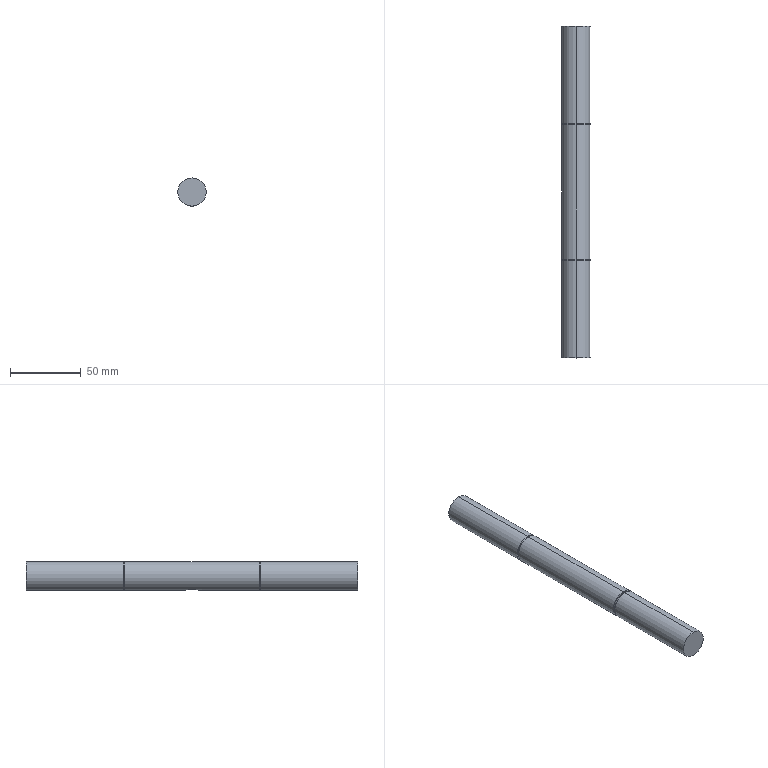Part | SolidWorks | features ICE 3, Chamfer 1, Extrusion 1 | 1 solid | 21 faces | box 20 x 235 x 20 mm | volume 73572 mm3 | cylinder 12 | plane 9 | commonest cylinder face diameters 20 x6 19 x4 6 x2
STEP:
#1=CARTESIAN_POINT('',(0.,235.,10.));
#2=VERTEX_POINT('',#1);
#3=CARTESIAN_POINT('',(0.,235.,-10.));
#4=VERTEX_POINT('',#3);
#5=CARTESIAN_POINT('',(0.,235.,0.));
#6=DIRECTION('',(0.,1.,0.));
#7=DIRECTION('',(0.,0.,1.));
#8=AXIS2_PLACEMENT_3D('',#5,#6,#7);
#9=CIRCLE('',#8,10.);
#10=EDGE_CURVE('',#2,#4,#9,.T.);
#11=ORIENTED_EDGE('',*,*,#10,.F.);
#12=CARTESIAN_POINT('',(0.,166.3,10.));
#13=VERTEX_POINT('',#12);
#14=CARTESIAN_POINT('',(0.,235.,10.));
#15=DIRECTION('',(0.,-1.,0.));
#16=VECTOR('',#15,1000.);
#17=LINE('',#14,#16);
#18=EDGE_CURVE('',#2,#13,#17,.T.);
#19=ORIENTED_EDGE('',*,*,#18,.T.);
#20=CARTESIAN_POINT('',(0.,166.3,-10.));
#21=VERTEX_POINT('',#20);
#22=CARTESIAN_POINT('',(0.,166.3,0.));
#23=DIRECTION('',(0.,1.,0.));
#24=DIRECTION('',(0.,0.,1.));
#25=AXIS2_PLACEMENT_3D('',#22,#23,#24);
#26=CIRCLE('',#25,10.);
#27=EDGE_CURVE('',#13,#21,#26,.T.);
#28=ORIENTED_EDGE('',*,*,#27,.T.);
#29=CARTESIAN_POINT('',(0.,235.,-10.));
#30=DIRECTION('',(0.,-1.,0.));
#31=VECTOR('',#30,1000.);
#32=LINE('',#29,#31);
#33=EDGE_CURVE('',#4,#21,#32,.T.);
#34=ORIENTED_EDGE('',*,*,#33,.F.);
#35=EDGE_LOOP('',(#11,#19,#28,#34));
#36=FACE_OUTER_BOUND('',#35,.T.);
#37=CARTESIAN_POINT('',(0.,235.,0.));
#38=DIRECTION('',(0.,-1.,0.));
#39=DIRECTION('',(0.,0.,-1.));
#40=AXIS2_PLACEMENT_3D('',#37,#38,#39);
#41=CYLINDRICAL_SURFACE('',#40,10.);
#42=ADVANCED_FACE('',(#36),#41,.T.);
#43=CARTESIAN_POINT('',(0.,166.3,9.5));
#44=VERTEX_POINT('',#43);
#45=CARTESIAN_POINT('',(0.,166.3,-9.5));
#46=VERTEX_POINT('',#45);
#47=CARTESIAN_POINT('',(0.,166.3,0.));
#48=DIRECTION('',(0.,1.,0.));
#49=DIRECTION('',(0.,0.,1.));
#50=AXIS2_PLACEMENT_3D('',#47,#48,#49);
#51=CIRCLE('',#50,9.5);
#52=EDGE_CURVE('',#44,#46,#51,.T.);
#53=ORIENTED_EDGE('',*,*,#52,.F.);
#54=CARTESIAN_POINT('',(0.,165.,9.5));
#55=VERTEX_POINT('',#54);
#56=CARTESIAN_POINT('',(0.,166.3,9.5));
#57=DIRECTION('',(0.,-1.,0.));
#58=VECTOR('',#57,1000.);
#59=LINE('',#56,#58);
#60=EDGE_CURVE('',#44,#55,#59,.T.);
#61=ORIENTED_EDGE('',*,*,#60,.T.);
#62=CARTESIAN_POINT('',(0.,165.,-9.5));
#63=VERTEX_POINT('',#62);
#64=CARTESIAN_POINT('',(0.,165.,0.));
#65=DIRECTION('',(0.,1.,0.));
#66=DIRECTION('',(0.,0.,1.));
#67=AXIS2_PLACEMENT_3D('',#64,#65,#66);
#68=CIRCLE('',#67,9.5);
#69=EDGE_CURVE('',#55,#63,#68,.T.);
#70=ORIENTED_EDGE('',*,*,#69,.T.);
#71=CARTESIAN_POINT('',(0.,166.3,-9.5));
#72=DIRECTION('',(0.,-1.,0.));
#73=VECTOR('',#72,1000.);
#74=LINE('',#71,#73);
#75=EDGE_CURVE('',#46,#63,#74,.T.);
#76=ORIENTED_EDGE('',*,*,#75,.F.);
#77=EDGE_LOOP('',(#53,#61,#70,#76));
#78=FACE_OUTER_BOUND('',#77,.T.);
#79=CARTESIAN_POINT('',(0.,166.3,0.));
#80=DIRECTION('',(0.,-1.,0.));
#81=DIRECTION('',(0.,0.,-1.));
#82=AXIS2_PLACEMENT_3D('',#79,#80,#81);
#83=CYLINDRICAL_SURFACE('',#82,9.5);
#84=ADVANCED_FACE('',(#78),#83,.T.);
#85=CARTESIAN_POINT('',(0.,68.7,-9.5));
#86=VERTEX_POINT('',#85);
#87=CARTESIAN_POINT('',(0.,68.7,9.5));
#88=VERTEX_POINT('',#87);
#89=CARTESIAN_POINT('',(0.,68.7,0.));
#90=DIRECTION('',(0.,-1.,0.));
#91=DIRECTION('',(0.,0.,-1.));
#92=AXIS2_PLACEMENT_3D('',#89,#90,#91);
#93=CIRCLE('',#92,9.5);
#94=EDGE_CURVE('',#86,#88,#93,.T.);
#95=ORIENTED_EDGE('',*,*,#94,.F.);
#96=CARTESIAN_POINT('',(0.,70.,-9.5));
#97=VERTEX_POINT('',#96);
#98=CARTESIAN_POINT('',(0.,68.7,-9.5));
#99=DIRECTION('',(0.,1.,0.));
#100=VECTOR('',#99,1000.);
#101=LINE('',#98,#100);
#102=EDGE_CURVE('',#86,#97,#101,.T.);
#103=ORIENTED_EDGE('',*,*,#102,.T.);
#104=CARTESIAN_POINT('',(0.,70.,9.5));
#105=VERTEX_POINT('',#104);
#106=CARTESIAN_POINT('',(0.,70.,0.));
#107=DIRECTION('',(0.,-1.,0.));
#108=DIRECTION('',(0.,0.,-1.));
#109=AXIS2_PLACEMENT_3D('',#106,#107,#108);
#110=CIRCLE('',#109,9.5);
#111=EDGE_CURVE('',#97,#105,#110,.T.);
#112=ORIENTED_EDGE('',*,*,#111,.T.);
#113=CARTESIAN_POINT('',(0.,68.7,9.5));
#114=DIRECTION('',(0.,1.,0.));
#115=VECTOR('',#114,1000.);
#116=LINE('',#113,#115);
#117=EDGE_CURVE('',#88,#105,#116,.T.);
#118=ORIENTED_EDGE('',*,*,#117,.F.);
#119=EDGE_LOOP('',(#95,#103,#112,#118));
#120=FACE_OUTER_BOUND('',#119,.T.);
#121=CARTESIAN_POINT('',(0.,68.7,0.));
#122=DIRECTION('',(0.,1.,0.));
#123=DIRECTION('',(0.,0.,1.));
#124=AXIS2_PLACEMENT_3D('',#121,#122,#123);
#125=CYLINDRICAL_SURFACE('',#124,9.5);
#126=ADVANCED_FACE('',(#120),#125,.T.);
#127=CARTESIAN_POINT('',(0.,68.7,-10.));
#128=VERTEX_POINT('',#127);
#129=CARTESIAN_POINT('',(0.,68.7,10.));
#130=VERTEX_POINT('',#129);
#131=CARTESIAN_POINT('',(0.,68.7,0.));
#132=DIRECTION('',(0.,-1.,0.));
#133=DIRECTION('',(0.,0.,-1.));
#134=AXIS2_PLACEMENT_3D('',#131,#132,#133);
#135=CIRCLE('',#134,10.);
#136=EDGE_CURVE('',#128,#130,#135,.T.);
#137=ORIENTED_EDGE('',*,*,#136,.T.);
#138=CARTESIAN_POINT('',(0.,0.,10.));
#139=VERTEX_POINT('',#138);
#140=CARTESIAN_POINT('',(0.,235.,10.));
#141=DIRECTION('',(0.,-1.,0.));
#142=VECTOR('',#141,1000.);
#143=LINE('',#140,#142);
#144=EDGE_CURVE('',#130,#139,#143,.T.);
#145=ORIENTED_EDGE('',*,*,#144,.T.);
#146=CARTESIAN_POINT('',(0.,0.,-10.));
#147=VERTEX_POINT('',#146);
#148=CARTESIAN_POINT('',(0.,0.,0.));
#149=DIRECTION('',(0.,1.,0.));
#150=DIRECTION('',(0.,0.,1.));
#151=AXIS2_PLACEMENT_3D('',#148,#149,#150);
#152=CIRCLE('',#151,10.);
#153=EDGE_CURVE('',#139,#147,#152,.T.);
#154=ORIENTED_EDGE('',*,*,#153,.T.);
#155=CARTESIAN_POINT('',(0.,235.,-10.));
#156=DIRECTION('',(0.,-1.,0.));
#157=VECTOR('',#156,1000.);
#158=LINE('',#155,#157);
#159=EDGE_CURVE('',#128,#147,#158,.T.);
#160=ORIENTED_EDGE('',*,*,#159,.F.);
#161=EDGE_LOOP('',(#137,#145,#154,#160));
#162=FACE_OUTER_BOUND('',#161,.T.);
#163=CARTESIAN_POINT('',(0.,235.,0.));
#164=DIRECTION('',(0.,-1.,0.));
#165=DIRECTION('',(0.,0.,-1.));
#166=AXIS2_PLACEMENT_3D('',#163,#164,#165);
#167=CYLINDRICAL_SURFACE('',#166,10.);
#168=ADVANCED_FACE('',(#162),#167,.T.);
#169=CARTESIAN_POINT('',(0.,165.,10.));
#170=VERTEX_POINT('',#169);
#171=CARTESIAN_POINT('',(0.,165.,-10.));
#172=VERTEX_POINT('',#171);
#173=CARTESIAN_POINT('',(0.,165.,0.));
#174=DIRECTION('',(0.,1.,0.));
#175=DIRECTION('',(0.,0.,1.));
#176=AXIS2_PLACEMENT_3D('',#173,#174,#175);
#177=CIRCLE('',#176,10.);
#178=EDGE_CURVE('',#170,#172,#177,.T.);
#179=ORIENTED_EDGE('',*,*,#178,.F.);
#180=CARTESIAN_POINT('',(0.,70.,10.));
#181=VERTEX_POINT('',#180);
#182=CARTESIAN_POINT('',(0.,235.,10.));
#183=DIRECTION('',(0.,-1.,0.));
#184=VECTOR('',#183,1000.);
#185=LINE('',#182,#184);
#186=EDGE_CURVE('',#170,#181,#185,.T.);
#187=ORIENTED_EDGE('',*,*,#186,.T.);
#188=CARTESIAN_POINT('',(0.,70.,-10.));
#189=VERTEX_POINT('',#188);
#190=CARTESIAN_POINT('',(0.,70.,0.));
#191=DIRECTION('',(0.,-1.,0.));
#192=DIRECTION('',(0.,0.,-1.));
#193=AXIS2_PLACEMENT_3D('',#190,#191,#192);
#194=CIRCLE('',#193,10.);
#195=EDGE_CURVE('',#189,#181,#194,.T.);
#196=ORIENTED_EDGE('',*,*,#195,.F.);
#197=CARTESIAN_POINT('',(0.,112.5,-10.));
#198=VERTEX_POINT('',#197);
#199=CARTESIAN_POINT('',(0.,235.,-10.));
#200=DIRECTION('',(0.,-1.,0.));
#201=VECTOR('',#200,1000.);
#202=LINE('',#199,#201);
#203=EDGE_CURVE('',#198,#189,#202,.T.);
#204=ORIENTED_EDGE('',*,*,#203,.F.);
#205=CARTESIAN_POINT('',(3.,115.5,-9.539));
#206=VERTEX_POINT('',#205);
#207=CARTESIAN_POINT('',(0.,112.5,-10.));
#208=CARTESIAN_POINT('',(0.1968,112.5,-10.));
#209=CARTESIAN_POINT('',(0.3967,112.52,-9.994));
#210=CARTESIAN_POINT('',(0.7821,112.597,-9.971));
#211=CARTESIAN_POINT('',(0.9695,112.654,-9.955));
#212=CARTESIAN_POINT('',(1.334,112.806,-9.912));
#213=CARTESIAN_POINT('',(1.507,112.899,-9.887));
#214=CARTESIAN_POINT('',(1.831,113.116,-9.832));
#215=CARTESIAN_POINT('',(1.983,113.241,-9.802));
#216=CARTESIAN_POINT('',(2.26,113.517,-9.742));
#217=CARTESIAN_POINT('',(2.383,113.667,-9.713));
#218=CARTESIAN_POINT('',(2.6,113.991,-9.657));
#219=CARTESIAN_POINT('',(2.694,114.167,-9.63));
#220=CARTESIAN_POINT('',(2.845,114.528,-9.587));
#221=CARTESIAN_POINT('',(2.902,114.715,-9.57));
#222=CARTESIAN_POINT('',(2.98,115.101,-9.546));
#223=CARTESIAN_POINT('',(3.,115.301,-9.539));
#224=CARTESIAN_POINT('',(3.,115.5,-9.539));
#225=B_SPLINE_CURVE_WITH_KNOTS('',3,(#207,#208,#209,#210,#211,#212,#213,#214,#215,#216,#217,#218,#219,#220,#221,#222,#223,#224),.UNSPECIFIED.,.F.,.F.,(4,2,2,2,2,2,2,2,4),(0.004718,0.005307,0.005896,0.006485,0.007074,0.007663,0.008252,0.008842,0.009431),.UNSPECIFIED.);
#226=EDGE_CURVE('',#198,#206,#225,.T.);
#227=ORIENTED_EDGE('',*,*,#226,.T.);
#228=CARTESIAN_POINT('',(3.,119.5,-9.539));
#229=VERTEX_POINT('',#228);
#230=CARTESIAN_POINT('',(3.,235.,-9.539));
#231=DIRECTION('',(0.,1.,0.));
#232=VECTOR('',#231,1000.);
#233=LINE('',#230,#232);
#234=EDGE_CURVE('',#206,#229,#233,.T.);
#235=ORIENTED_EDGE('',*,*,#234,.T.);
#236=CARTESIAN_POINT('',(0.,122.5,-10.));
#237=VERTEX_POINT('',#236);
#238=CARTESIAN_POINT('',(3.,119.5,-9.539));
#239=CARTESIAN_POINT('',(3.,119.7,-9.539));
#240=CARTESIAN_POINT('',(2.98,119.895,-9.546));
#241=CARTESIAN_POINT('',(2.903,120.281,-9.569));
#242=CARTESIAN_POINT('',(2.845,120.472,-9.587));
#243=CARTESIAN_POINT('',(2.694,120.835,-9.631));
#244=CARTESIAN_POINT('',(2.602,121.006,-9.656));
#245=CARTESIAN_POINT('',(2.384,121.332,-9.712));
#246=CARTESIAN_POINT('',(2.258,121.485,-9.743));
#247=CARTESIAN_POINT('',(1.845,121.897,-9.832));
#248=CARTESIAN_POINT('',(1.512,122.12,-9.892));
#249=CARTESIAN_POINT('',(0.971,122.345,-9.954));
#250=CARTESIAN_POINT('',(0.7806,122.403,-9.971));
#251=CARTESIAN_POINT('',(0.3926,122.481,-9.994));
#252=CARTESIAN_POINT('',(0.197,122.5,-10.));
#253=CARTESIAN_POINT('',(0.,122.5,-10.));
#254=B_SPLINE_CURVE_WITH_KNOTS('',3,(#238,#239,#240,#241,#242,#243,#244,#245,#246,#247,#248,#249,#250,#251,#252,#253),.UNSPECIFIED.,.F.,.F.,(4,2,2,2,2,2,2,4),(0.,0.0005898,0.00118,0.001769,0.002359,0.003539,0.004128,0.004718),.UNSPECIFIED.);
#255=EDGE_CURVE('',#229,#237,#254,.T.);
#256=ORIENTED_EDGE('',*,*,#255,.T.);
#257=CARTESIAN_POINT('',(0.,235.,-10.));
#258=DIRECTION('',(0.,-1.,0.));
#259=VECTOR('',#258,1000.);
#260=LINE('',#257,#259);
#261=EDGE_CURVE('',#172,#237,#260,.T.);
#262=ORIENTED_EDGE('',*,*,#261,.F.);
#263=EDGE_LOOP('',(#179,#187,#196,#204,#227,#235,#256,#262));
#264=FACE_OUTER_BOUND('',#263,.T.);
#265=CARTESIAN_POINT('',(0.,235.,0.));
#266=DIRECTION('',(0.,-1.,0.));
#267=DIRECTION('',(0.,0.,-1.));
#268=AXIS2_PLACEMENT_3D('',#265,#266,#267);
#269=CYLINDRICAL_SURFACE('',#268,10.);
#270=ADVANCED_FACE('',(#264),#269,.T.);
#271=ORIENTED_EDGE('',*,*,#186,.F.);
#272=CARTESIAN_POINT('',(0.,165.,0.));
#273=DIRECTION('',(0.,1.,0.));
#274=DIRECTION('',(0.,0.,1.));
#275=AXIS2_PLACEMENT_3D('',#272,#273,#274);
#276=CIRCLE('',#275,10.);
#277=EDGE_CURVE('',#172,#170,#276,.T.);
#278=ORIENTED_EDGE('',*,*,#277,.F.);
#279=ORIENTED_EDGE('',*,*,#261,.T.);
#280=CARTESIAN_POINT('',(-3.,119.5,-9.539));
#281=VERTEX_POINT('',#280);
#282=CARTESIAN_POINT('',(0.,122.5,-10.));
#283=CARTESIAN_POINT('',(-0.1968,122.5,-10.));
#284=CARTESIAN_POINT('',(-0.3967,122.48,-9.994));
#285=CARTESIAN_POINT('',(-0.7821,122.403,-9.971));
#286=CARTESIAN_POINT('',(-0.9695,122.346,-9.955));
#287=CARTESIAN_POINT('',(-1.334,122.194,-9.912));
#288=CARTESIAN_POINT('',(-1.507,122.101,-9.887));
#289=CARTESIAN_POINT('',(-1.831,121.884,-9.832));
#290=CARTESIAN_POINT('',(-1.983,121.759,-9.802));
#291=CARTESIAN_POINT('',(-2.26,121.483,-9.742));
#292=CARTESIAN_POINT('',(-2.383,121.333,-9.713));
#293=CARTESIAN_POINT('',(-2.6,121.009,-9.657));
#294=CARTESIAN_POINT('',(-2.694,120.833,-9.63));
#295=CARTESIAN_POINT('',(-2.845,120.472,-9.587));
#296=CARTESIAN_POINT('',(-2.902,120.285,-9.57));
#297=CARTESIAN_POINT('',(-2.98,119.899,-9.546));
#298=CARTESIAN_POINT('',(-3.,119.699,-9.539));
#299=CARTESIAN_POINT('',(-3.,119.5,-9.539));
#300=B_SPLINE_CURVE_WITH_KNOTS('',3,(#282,#283,#284,#285,#286,#287,#288,#289,#290,#291,#292,#293,#294,#295,#296,#297,#298,#299),.UNSPECIFIED.,.F.,.F.,(4,2,2,2,2,2,2,2,4),(0.004718,0.005307,0.005896,0.006485,0.007074,0.007663,0.008252,0.008842,0.009431),.UNSPECIFIED.);
#301=EDGE_CURVE('',#237,#281,#300,.T.);
#302=ORIENTED_EDGE('',*,*,#301,.T.);
#303=CARTESIAN_POINT('',(-3.,115.5,-9.539));
#304=VERTEX_POINT('',#303);
#305=CARTESIAN_POINT('',(-3.,235.,-9.539));
#306=DIRECTION('',(0.,-1.,0.));
#307=VECTOR('',#306,1000.);
#308=LINE('',#305,#307);
#309=EDGE_CURVE('',#281,#304,#308,.T.);
#310=ORIENTED_EDGE('',*,*,#309,.T.);
#311=CARTESIAN_POINT('',(-3.,115.5,-9.539));
#312=CARTESIAN_POINT('',(-3.,115.3,-9.539));
#313=CARTESIAN_POINT('',(-2.98,115.105,-9.546));
#314=CARTESIAN_POINT('',(-2.903,114.719,-9.569));
#315=CARTESIAN_POINT('',(-2.845,114.528,-9.587));
#316=CARTESIAN_POINT('',(-2.694,114.165,-9.631));
#317=CARTESIAN_POINT('',(-2.602,113.994,-9.656));
#318=CARTESIAN_POINT('',(-2.384,113.668,-9.712));
#319=CARTESIAN_POINT('',(-2.258,113.515,-9.743));
#320=CARTESIAN_POINT('',(-1.845,113.103,-9.832));
#321=CARTESIAN_POINT('',(-1.512,112.88,-9.892));
#322=CARTESIAN_POINT('',(-0.971,112.655,-9.954));
#323=CARTESIAN_POINT('',(-0.7806,112.597,-9.971));
#324=CARTESIAN_POINT('',(-0.3926,112.519,-9.994));
#325=CARTESIAN_POINT('',(-0.197,112.5,-10.));
#326=CARTESIAN_POINT('',(0.,112.5,-10.));
#327=B_SPLINE_CURVE_WITH_KNOTS('',3,(#311,#312,#313,#314,#315,#316,#317,#318,#319,#320,#321,#322,#323,#324,#325,#326),.UNSPECIFIED.,.F.,.F.,(4,2,2,2,2,2,2,4),(0.,0.0005898,0.00118,0.001769,0.002359,0.003539,0.004128,0.004718),.UNSPECIFIED.);
#328=EDGE_CURVE('',#304,#198,#327,.T.);
#329=ORIENTED_EDGE('',*,*,#328,.T.);
#330=ORIENTED_EDGE('',*,*,#203,.T.);
#331=CARTESIAN_POINT('',(0.,70.,0.));
#332=DIRECTION('',(0.,-1.,0.));
#333=DIRECTION('',(0.,0.,-1.));
#334=AXIS2_PLACEMENT_3D('',#331,#332,#333);
#335=CIRCLE('',#334,10.);
#336=EDGE_CURVE('',#181,#189,#335,.T.);
#337=ORIENTED_EDGE('',*,*,#336,.F.);
#338=EDGE_LOOP('',(#271,#278,#279,#302,#310,#329,#330,#337));
#339=FACE_OUTER_BOUND('',#338,.T.);
#340=CARTESIAN_POINT('',(0.,235.,0.));
#341=DIRECTION('',(0.,-1.,0.));
#342=DIRECTION('',(0.,0.,-1.));
#343=AXIS2_PLACEMENT_3D('',#340,#341,#342);
#344=CYLINDRICAL_SURFACE('',#343,10.);
#345=ADVANCED_FACE('',(#339),#344,.T.);
#346=ORIENTED_EDGE('',*,*,#144,.F.);
#347=CARTESIAN_POINT('',(0.,68.7,0.));
#348=DIRECTION('',(0.,-1.,0.));
#349=DIRECTION('',(0.,0.,-1.));
#350=AXIS2_PLACEMENT_3D('',#347,#348,#349);
#351=CIRCLE('',#350,10.);
#352=EDGE_CURVE('',#130,#128,#351,.T.);
#353=ORIENTED_EDGE('',*,*,#352,.T.);
#354=ORIENTED_EDGE('',*,*,#159,.T.);
#355=CARTESIAN_POINT('',(0.,0.,0.));
#356=DIRECTION('',(0.,1.,0.));
#357=DIRECTION('',(0.,0.,1.));
#358=AXIS2_PLACEMENT_3D('',#355,#356,#357);
#359=CIRCLE('',#358,10.);
#360=EDGE_CURVE('',#147,#139,#359,.T.);
#361=ORIENTED_EDGE('',*,*,#360,.T.);
#362=EDGE_LOOP('',(#346,#353,#354,#361));
#363=FACE_OUTER_BOUND('',#362,.T.);
#364=CARTESIAN_POINT('',(0.,235.,0.));
#365=DIRECTION('',(0.,-1.,0.));
#366=DIRECTION('',(0.,0.,-1.));
#367=AXIS2_PLACEMENT_3D('',#364,#365,#366);
#368=CYLINDRICAL_SURFACE('',#367,10.);
#369=ADVANCED_FACE('',(#363),#368,.T.);
#370=ORIENTED_EDGE('',*,*,#360,.F.);
#371=ORIENTED_EDGE('',*,*,#153,.F.);
#372=EDGE_LOOP('',(#370,#371));
#373=FACE_OUTER_BOUND('',#372,.T.);
#374=CARTESIAN_POINT('',(0.,0.,0.));
#375=DIRECTION('',(0.,1.,0.));
#376=DIRECTION('',(0.,0.,1.));
#377=AXIS2_PLACEMENT_3D('',#374,#375,#376);
#378=PLANE('',#377);
#379=ADVANCED_FACE('',(#373),#378,.F.);
#380=ORIENTED_EDGE('',*,*,#136,.F.);
#381=ORIENTED_EDGE('',*,*,#352,.F.);
#382=EDGE_LOOP('',(#380,#381));
#383=FACE_OUTER_BOUND('',#382,.T.);
#384=CARTESIAN_POINT('',(0.,68.7,0.));
#385=DIRECTION('',(0.,-1.,0.));
#386=DIRECTION('',(0.,0.,-1.));
#387=AXIS2_PLACEMENT_3D('',#384,#385,#386);
#388=CIRCLE('',#387,9.5);
#389=EDGE_CURVE('',#88,#86,#388,.T.);
#390=ORIENTED_EDGE('',*,*,#389,.T.);
#391=ORIENTED_EDGE('',*,*,#94,.T.);
#392=EDGE_LOOP('',(#390,#391));
#393=FACE_BOUND('',#392,.T.);
#394=CARTESIAN_POINT('',(0.,68.7,0.));
#395=DIRECTION('',(0.,-1.,0.));
#396=DIRECTION('',(0.,0.,-1.));
#397=AXIS2_PLACEMENT_3D('',#394,#395,#396);
#398=PLANE('',#397);
#399=ADVANCED_FACE('',(#383,#393),#398,.F.);
#400=ORIENTED_EDGE('',*,*,#195,.T.);
#401=ORIENTED_EDGE('',*,*,#336,.T.);
#402=EDGE_LOOP('',(#400,#401));
#403=FACE_OUTER_BOUND('',#402,.T.);
#404=CARTESIAN_POINT('',(0.,70.,0.));
#405=DIRECTION('',(0.,-1.,0.));
#406=DIRECTION('',(0.,0.,-1.));
#407=AXIS2_PLACEMENT_3D('',#404,#405,#406);
#408=CIRCLE('',#407,9.5);
#409=EDGE_CURVE('',#105,#97,#408,.T.);
#410=ORIENTED_EDGE('',*,*,#409,.F.);
#411=ORIENTED_EDGE('',*,*,#111,.F.);
#412=EDGE_LOOP('',(#410,#411));
#413=FACE_BOUND('',#412,.T.);
#414=CARTESIAN_POINT('',(0.,70.,0.));
#415=DIRECTION('',(0.,-1.,0.));
#416=DIRECTION('',(0.,0.,-1.));
#417=AXIS2_PLACEMENT_3D('',#414,#415,#416);
#418=PLANE('',#417);
#419=ADVANCED_FACE('',(#403,#413),#418,.T.);
#420=ORIENTED_EDGE('',*,*,#102,.F.);
#421=ORIENTED_EDGE('',*,*,#389,.F.);
#422=ORIENTED_EDGE('',*,*,#117,.T.);
#423=ORIENTED_EDGE('',*,*,#409,.T.);
#424=EDGE_LOOP('',(#420,#421,#422,#423));
#425=FACE_OUTER_BOUND('',#424,.T.);
#426=CARTESIAN_POINT('',(0.,68.7,0.));
#427=DIRECTION('',(0.,1.,0.));
#428=DIRECTION('',(0.,0.,1.));
#429=AXIS2_PLACEMENT_3D('',#426,#427,#428);
#430=CYLINDRICAL_SURFACE('',#429,9.5);
#431=ADVANCED_FACE('',(#425),#430,.T.);
#432=CARTESIAN_POINT('',(0.,166.3,0.));
#433=DIRECTION('',(0.,1.,0.));
#434=DIRECTION('',(0.,0.,1.));
#435=AXIS2_PLACEMENT_3D('',#432,#433,#434);
#436=CIRCLE('',#435,10.);
#437=EDGE_CURVE('',#21,#13,#436,.T.);
#438=ORIENTED_EDGE('',*,*,#437,.F.);
#439=ORIENTED_EDGE('',*,*,#27,.F.);
#440=EDGE_LOOP('',(#438,#439));
#441=FACE_OUTER_BOUND('',#440,.T.);
#442=CARTESIAN_POINT('',(0.,166.3,0.));
#443=DIRECTION('',(0.,1.,0.));
#444=DIRECTION('',(0.,0.,1.));
#445=AXIS2_PLACEMENT_3D('',#442,#443,#444);
#446=CIRCLE('',#445,9.5);
#447=EDGE_CURVE('',#46,#44,#446,.T.);
#448=ORIENTED_EDGE('',*,*,#447,.T.);
#449=ORIENTED_EDGE('',*,*,#52,.T.);
#450=EDGE_LOOP('',(#448,#449));
#451=FACE_BOUND('',#450,.T.);
#452=CARTESIAN_POINT('',(0.,166.3,0.));
#453=DIRECTION('',(0.,1.,0.));
#454=DIRECTION('',(0.,0.,1.));
#455=AXIS2_PLACEMENT_3D('',#452,#453,#454);
#456=PLANE('',#455);
#457=ADVANCED_FACE('',(#441,#451),#456,.F.);
#458=ORIENTED_EDGE('',*,*,#277,.T.);
#459=ORIENTED_EDGE('',*,*,#178,.T.);
#460=EDGE_LOOP('',(#458,#459));
#461=FACE_OUTER_BOUND('',#460,.T.);
#462=CARTESIAN_POINT('',(0.,165.,0.));
#463=DIRECTION('',(0.,1.,0.));
#464=DIRECTION('',(0.,0.,1.));
#465=AXIS2_PLACEMENT_3D('',#462,#463,#464);
#466=CIRCLE('',#465,9.5);
#467=EDGE_CURVE('',#63,#55,#466,.T.);
#468=ORIENTED_EDGE('',*,*,#467,.F.);
#469=ORIENTED_EDGE('',*,*,#69,.F.);
#470=EDGE_LOOP('',(#468,#469));
#471=FACE_BOUND('',#470,.T.);
#472=CARTESIAN_POINT('',(0.,165.,0.));
#473=DIRECTION('',(0.,1.,0.));
#474=DIRECTION('',(0.,0.,1.));
#475=AXIS2_PLACEMENT_3D('',#472,#473,#474);
#476=PLANE('',#475);
#477=ADVANCED_FACE('',(#461,#471),#476,.T.);
#478=ORIENTED_EDGE('',*,*,#60,.F.);
#479=ORIENTED_EDGE('',*,*,#447,.F.);
#480=ORIENTED_EDGE('',*,*,#75,.T.);
#481=ORIENTED_EDGE('',*,*,#467,.T.);
#482=EDGE_LOOP('',(#478,#479,#480,#481));
#483=FACE_OUTER_BOUND('',#482,.T.);
#484=CARTESIAN_POINT('',(0.,166.3,0.));
#485=DIRECTION('',(0.,-1.,0.));
#486=DIRECTION('',(0.,0.,-1.));
#487=AXIS2_PLACEMENT_3D('',#484,#485,#486);
#488=CYLINDRICAL_SURFACE('',#487,9.5);
#489=ADVANCED_FACE('',(#483),#488,.T.);
#490=CARTESIAN_POINT('',(0.,235.,0.));
#491=DIRECTION('',(0.,1.,0.));
#492=DIRECTION('',(0.,0.,1.));
#493=AXIS2_PLACEMENT_3D('',#490,#491,#492);
#494=CIRCLE('',#493,10.);
#495=EDGE_CURVE('',#4,#2,#494,.T.);
#496=ORIENTED_EDGE('',*,*,#495,.T.);
#497=ORIENTED_EDGE('',*,*,#10,.T.);
#498=EDGE_LOOP('',(#496,#497));
#499=FACE_OUTER_BOUND('',#498,.T.);
#500=CARTESIAN_POINT('',(0.,235.,0.));
#501=DIRECTION('',(0.,1.,0.));
#502=DIRECTION('',(0.,0.,1.));
#503=AXIS2_PLACEMENT_3D('',#500,#501,#502);
#504=PLANE('',#503);
#505=ADVANCED_FACE('',(#499),#504,.T.);
#506=ORIENTED_EDGE('',*,*,#18,.F.);
#507=ORIENTED_EDGE('',*,*,#495,.F.);
#508=ORIENTED_EDGE('',*,*,#33,.T.);
#509=ORIENTED_EDGE('',*,*,#437,.T.);
#510=EDGE_LOOP('',(#506,#507,#508,#509));
#511=FACE_OUTER_BOUND('',#510,.T.);
#512=CARTESIAN_POINT('',(0.,235.,0.));
#513=DIRECTION('',(0.,-1.,0.));
#514=DIRECTION('',(0.,0.,-1.));
#515=AXIS2_PLACEMENT_3D('',#512,#513,#514);
#516=CYLINDRICAL_SURFACE('',#515,10.);
#517=ADVANCED_FACE('',(#511),#516,.T.);
#518=CARTESIAN_POINT('',(-3.,115.5,-6.5));
#519=VERTEX_POINT('',#518);
#520=CARTESIAN_POINT('',(-3.,115.5,-6.5));
#521=DIRECTION('',(0.,0.,-1.));
#522=VECTOR('',#521,1000.);
#523=LINE('',#520,#522);
#524=EDGE_CURVE('',#519,#304,#523,.T.);
#525=ORIENTED_EDGE('',*,*,#524,.F.);
#526=CARTESIAN_POINT('',(3.,115.5,-6.5));
#527=VERTEX_POINT('',#526);
#528=CARTESIAN_POINT('',(0.,115.5,-6.5));
#529=DIRECTION('',(0.,0.,-1.));
#530=DIRECTION('',(-1.,0.,0.));
#531=AXIS2_PLACEMENT_3D('',#528,#529,#530);
#532=CIRCLE('',#531,3.);
#533=EDGE_CURVE('',#527,#519,#532,.T.);
#534=ORIENTED_EDGE('',*,*,#533,.F.);
#535=CARTESIAN_POINT('',(3.,115.5,-6.5));
#536=DIRECTION('',(0.,0.,-1.));
#537=VECTOR('',#536,1000.);
#538=LINE('',#535,#537);
#539=EDGE_CURVE('',#527,#206,#538,.T.);
#540=ORIENTED_EDGE('',*,*,#539,.T.);
#541=ORIENTED_EDGE('',*,*,#226,.F.);
#542=ORIENTED_EDGE('',*,*,#328,.F.);
#543=EDGE_LOOP('',(#525,#534,#540,#541,#542));
#544=FACE_OUTER_BOUND('',#543,.T.);
#545=CARTESIAN_POINT('',(0.,115.5,-6.5));
#546=DIRECTION('',(0.,0.,-1.));
#547=DIRECTION('',(-1.,0.,0.));
#548=AXIS2_PLACEMENT_3D('',#545,#546,#547);
#549=CYLINDRICAL_SURFACE('',#548,3.);
#550=ADVANCED_FACE('',(#544),#549,.F.);
#551=ORIENTED_EDGE('',*,*,#539,.F.);
#552=CARTESIAN_POINT('',(3.,119.5,-6.5));
#553=VERTEX_POINT('',#552);
#554=CARTESIAN_POINT('',(3.,115.5,-6.5));
#555=DIRECTION('',(0.,-1.,0.));
#556=VECTOR('',#555,1000.);
#557=LINE('',#554,#556);
#558=EDGE_CURVE('',#553,#527,#557,.T.);
#559=ORIENTED_EDGE('',*,*,#558,.F.);
#560=CARTESIAN_POINT('',(3.,119.5,-6.5));
#561=DIRECTION('',(0.,0.,-1.));
#562=VECTOR('',#561,1000.);
#563=LINE('',#560,#562);
#564=EDGE_CURVE('',#553,#229,#563,.T.);
#565=ORIENTED_EDGE('',*,*,#564,.T.);
#566=ORIENTED_EDGE('',*,*,#234,.F.);
#567=EDGE_LOOP('',(#551,#559,#565,#566));
#568=FACE_OUTER_BOUND('',#567,.T.);
#569=CARTESIAN_POINT('',(3.,115.5,-6.5));
#570=DIRECTION('',(1.,0.,0.));
#571=DIRECTION('',(0.,0.,-1.));
#572=AXIS2_PLACEMENT_3D('',#569,#570,#571);
#573=PLANE('',#572);
#574=ADVANCED_FACE('',(#568),#573,.F.);
#575=ORIENTED_EDGE('',*,*,#564,.F.);
#576=CARTESIAN_POINT('',(-3.,119.5,-6.5));
#577=VERTEX_POINT('',#576);
#578=CARTESIAN_POINT('',(0.,119.5,-6.5));
#579=DIRECTION('',(0.,0.,-1.));
#580=DIRECTION('',(-1.,0.,0.));
#581=AXIS2_PLACEMENT_3D('',#578,#579,#580);
#582=CIRCLE('',#581,3.);
#583=EDGE_CURVE('',#577,#553,#582,.T.);
#584=ORIENTED_EDGE('',*,*,#583,.F.);
#585=CARTESIAN_POINT('',(-3.,119.5,-6.5));
#586=DIRECTION('',(0.,0.,-1.));
#587=VECTOR('',#586,1000.);
#588=LINE('',#585,#587);
#589=EDGE_CURVE('',#577,#281,#588,.T.);
#590=ORIENTED_EDGE('',*,*,#589,.T.);
#591=ORIENTED_EDGE('',*,*,#301,.F.);
#592=ORIENTED_EDGE('',*,*,#255,.F.);
#593=EDGE_LOOP('',(#575,#584,#590,#591,#592));
#594=FACE_OUTER_BOUND('',#593,.T.);
#595=CARTESIAN_POINT('',(0.,119.5,-6.5));
#596=DIRECTION('',(0.,0.,-1.));
#597=DIRECTION('',(-1.,0.,0.));
#598=AXIS2_PLACEMENT_3D('',#595,#596,#597);
#599=CYLINDRICAL_SURFACE('',#598,3.);
#600=ADVANCED_FACE('',(#594),#599,.F.);
#601=ORIENTED_EDGE('',*,*,#589,.F.);
#602=CARTESIAN_POINT('',(-3.,115.5,-6.5));
#603=DIRECTION('',(0.,1.,0.));
#604=VECTOR('',#603,1000.);
#605=LINE('',#602,#604);
#606=EDGE_CURVE('',#519,#577,#605,.T.);
#607=ORIENTED_EDGE('',*,*,#606,.F.);
#608=ORIENTED_EDGE('',*,*,#524,.T.);
#609=ORIENTED_EDGE('',*,*,#309,.F.);
#610=EDGE_LOOP('',(#601,#607,#608,#609));
#611=FACE_OUTER_BOUND('',#610,.T.);
#612=CARTESIAN_POINT('',(-3.,115.5,-6.5));
#613=DIRECTION('',(-1.,0.,0.));
#614=DIRECTION('',(0.,0.,1.));
#615=AXIS2_PLACEMENT_3D('',#612,#613,#614);
#616=PLANE('',#615);
#617=ADVANCED_FACE('',(#611),#616,.F.);
#618=ORIENTED_EDGE('',*,*,#533,.T.);
#619=ORIENTED_EDGE('',*,*,#606,.T.);
#620=ORIENTED_EDGE('',*,*,#583,.T.);
#621=ORIENTED_EDGE('',*,*,#558,.T.);
#622=EDGE_LOOP('',(#618,#619,#620,#621));
#623=FACE_OUTER_BOUND('',#622,.T.);
#624=CARTESIAN_POINT('',(0.,115.5,-6.5));
#625=DIRECTION('',(0.,0.,-1.));
#626=DIRECTION('',(-1.,0.,0.));
#627=AXIS2_PLACEMENT_3D('',#624,#625,#626);
#628=PLANE('',#627);
#629=ADVANCED_FACE('',(#623),#628,.T.);
#630=CLOSED_SHELL('',(#42,#84,#126,#168,#270,#345,#369,#379,#399,#419,#431,#457,#477,#489,#505,#517,#550,#574,#600,#617,#629));
#631=MANIFOLD_SOLID_BREP('',#630);
#632=CARTESIAN_POINT('',(0.,0.,0.));
#633=DIRECTION('',(0.,0.,1.));
#634=DIRECTION('',(1.,0.,0.));
#635=AXIS2_PLACEMENT_3D('',#632,#633,#634);
#636=(LENGTH_UNIT()NAMED_UNIT(*)SI_UNIT(.MILLI.,.METRE.));
#637=UNCERTAINTY_MEASURE_WITH_UNIT(LENGTH_MEASURE(0.00001),#636,'','');
#638=(NAMED_UNIT(*)PLANE_ANGLE_UNIT()SI_UNIT($,.RADIAN.));
#639=(NAMED_UNIT(*)SI_UNIT($,.STERADIAN.)SOLID_ANGLE_UNIT());
#640=(GEOMETRIC_REPRESENTATION_CONTEXT(3)GLOBAL_UNCERTAINTY_ASSIGNED_CONTEXT((#637))GLOBAL_UNIT_ASSIGNED_CONTEXT((#636,#638,#639))REPRESENTATION_CONTEXT('',''));
#641=ADVANCED_BREP_SHAPE_REPRESENTATION('',(#631,#635),#640);